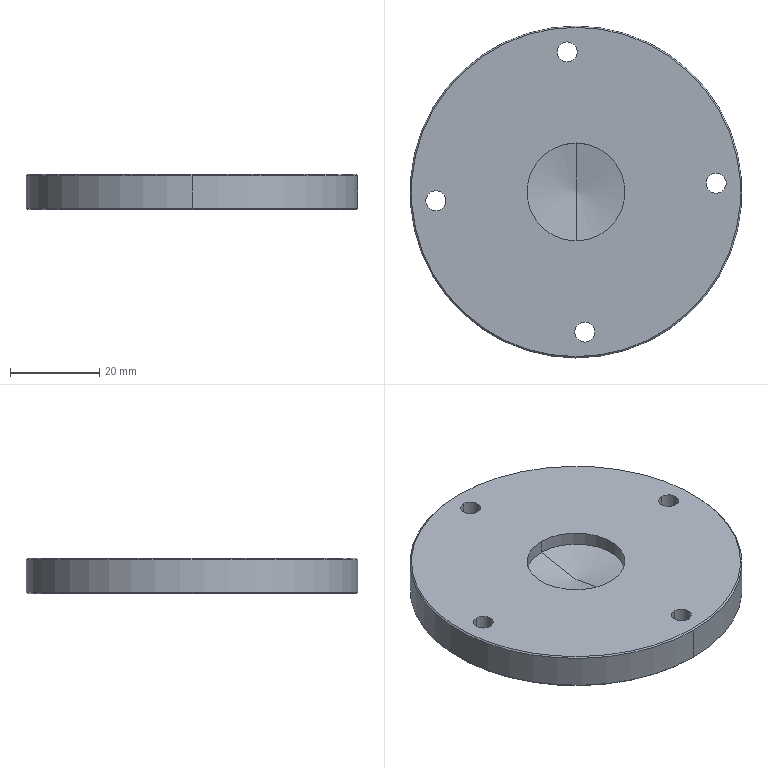Part | SolidWorks | features BaseBody 1 | 1 solid | 32 faces | box 74.5 x 74.5 x 8 mm | volume 32380 mm3 | cylinder 20 | cone 6 | plane 6 | commonest cylinder face diameters 4.5 x8 8 x8 22 x2 74.5 x2
STEP:
#1=CARTESIAN_POINT('',(560.081,-185.625,38.889));
#2=VERTEX_POINT('',#1);
#3=CARTESIAN_POINT('',(560.081,-193.625,38.889));
#4=VERTEX_POINT('',#3);
#5=CARTESIAN_POINT('',(560.081,-189.625,38.889));
#6=DIRECTION('',(0.,-0.000000003,1.));
#7=DIRECTION('',(0.,-1.,-0.000000003));
#8=AXIS2_PLACEMENT_3D('',#5,#6,#7);
#9=CIRCLE('',#8,4.);
#10=EDGE_CURVE('',#2,#4,#9,.T.);
#11=ORIENTED_EDGE('',*,*,#10,.F.);
#12=CARTESIAN_POINT('',(560.081,-185.625,43.089));
#13=VERTEX_POINT('',#12);
#14=CARTESIAN_POINT('',(560.081,-185.625,38.889));
#15=DIRECTION('',(0.,-0.000000003,1.));
#16=VECTOR('',#15,1000.);
#17=LINE('',#14,#16);
#18=EDGE_CURVE('',#2,#13,#17,.T.);
#19=ORIENTED_EDGE('',*,*,#18,.T.);
#20=CARTESIAN_POINT('',(560.081,-193.625,43.089));
#21=VERTEX_POINT('',#20);
#22=CARTESIAN_POINT('',(560.081,-189.625,43.089));
#23=DIRECTION('',(0.,0.000000003,-1.));
#24=DIRECTION('',(0.,-1.,-0.000000003));
#25=AXIS2_PLACEMENT_3D('',#22,#23,#24);
#26=CIRCLE('',#25,4.);
#27=EDGE_CURVE('',#21,#13,#26,.T.);
#28=ORIENTED_EDGE('',*,*,#27,.F.);
#29=CARTESIAN_POINT('',(560.081,-193.625,38.889));
#30=DIRECTION('',(0.,-0.000000003,1.));
#31=VECTOR('',#30,1000.);
#32=LINE('',#29,#31);
#33=EDGE_CURVE('',#4,#21,#32,.T.);
#34=ORIENTED_EDGE('',*,*,#33,.F.);
#35=EDGE_LOOP('',(#11,#19,#28,#34));
#36=FACE_OUTER_BOUND('',#35,.T.);
#37=CARTESIAN_POINT('',(560.081,-189.625,38.889));
#38=DIRECTION('',(0.,-0.000000003,1.));
#39=DIRECTION('',(0.,-1.,-0.000000003));
#40=AXIS2_PLACEMENT_3D('',#37,#38,#39);
#41=CYLINDRICAL_SURFACE('',#40,4.);
#42=ADVANCED_FACE('',(#36),#41,.F.);
#43=CARTESIAN_POINT('',(593.495,-215.086,38.889));
#44=VERTEX_POINT('',#43);
#45=CARTESIAN_POINT('',(593.495,-223.086,38.889));
#46=VERTEX_POINT('',#45);
#47=CARTESIAN_POINT('',(593.495,-219.086,38.889));
#48=DIRECTION('',(0.,-0.000000003,1.));
#49=DIRECTION('',(0.,-1.,-0.000000003));
#50=AXIS2_PLACEMENT_3D('',#47,#48,#49);
#51=CIRCLE('',#50,4.);
#52=EDGE_CURVE('',#44,#46,#51,.T.);
#53=ORIENTED_EDGE('',*,*,#52,.F.);
#54=CARTESIAN_POINT('',(593.495,-215.086,43.089));
#55=VERTEX_POINT('',#54);
#56=CARTESIAN_POINT('',(593.495,-215.086,38.889));
#57=DIRECTION('',(0.,-0.000000003,1.));
#58=VECTOR('',#57,1000.);
#59=LINE('',#56,#58);
#60=EDGE_CURVE('',#44,#55,#59,.T.);
#61=ORIENTED_EDGE('',*,*,#60,.T.);
#62=CARTESIAN_POINT('',(593.495,-223.086,43.089));
#63=VERTEX_POINT('',#62);
#64=CARTESIAN_POINT('',(593.495,-219.086,43.089));
#65=DIRECTION('',(0.,0.000000003,-1.));
#66=DIRECTION('',(0.,-1.,-0.000000003));
#67=AXIS2_PLACEMENT_3D('',#64,#65,#66);
#68=CIRCLE('',#67,4.);
#69=EDGE_CURVE('',#63,#55,#68,.T.);
#70=ORIENTED_EDGE('',*,*,#69,.F.);
#71=CARTESIAN_POINT('',(593.495,-223.086,38.889));
#72=DIRECTION('',(0.,-0.000000003,1.));
#73=VECTOR('',#72,1000.);
#74=LINE('',#71,#73);
#75=EDGE_CURVE('',#46,#63,#74,.T.);
#76=ORIENTED_EDGE('',*,*,#75,.F.);
#77=EDGE_LOOP('',(#53,#61,#70,#76));
#78=FACE_OUTER_BOUND('',#77,.T.);
#79=CARTESIAN_POINT('',(593.495,-219.086,38.889));
#80=DIRECTION('',(0.,-0.000000003,1.));
#81=DIRECTION('',(0.,-1.,-0.000000003));
#82=AXIS2_PLACEMENT_3D('',#79,#80,#81);
#83=CYLINDRICAL_SURFACE('',#82,4.);
#84=ADVANCED_FACE('',(#78),#83,.F.);
#85=CARTESIAN_POINT('',(622.957,-181.672,38.889));
#86=VERTEX_POINT('',#85);
#87=CARTESIAN_POINT('',(622.957,-189.672,38.889));
#88=VERTEX_POINT('',#87);
#89=CARTESIAN_POINT('',(622.957,-185.672,38.889));
#90=DIRECTION('',(0.,-0.000000003,1.));
#91=DIRECTION('',(0.,-1.,-0.000000003));
#92=AXIS2_PLACEMENT_3D('',#89,#90,#91);
#93=CIRCLE('',#92,4.);
#94=EDGE_CURVE('',#86,#88,#93,.T.);
#95=ORIENTED_EDGE('',*,*,#94,.F.);
#96=CARTESIAN_POINT('',(622.957,-181.672,43.089));
#97=VERTEX_POINT('',#96);
#98=CARTESIAN_POINT('',(622.957,-181.672,38.889));
#99=DIRECTION('',(0.,-0.000000003,1.));
#100=VECTOR('',#99,1000.);
#101=LINE('',#98,#100);
#102=EDGE_CURVE('',#86,#97,#101,.T.);
#103=ORIENTED_EDGE('',*,*,#102,.T.);
#104=CARTESIAN_POINT('',(622.957,-189.672,43.089));
#105=VERTEX_POINT('',#104);
#106=CARTESIAN_POINT('',(622.957,-185.672,43.089));
#107=DIRECTION('',(0.,0.000000003,-1.));
#108=DIRECTION('',(0.,-1.,-0.000000003));
#109=AXIS2_PLACEMENT_3D('',#106,#107,#108);
#110=CIRCLE('',#109,4.);
#111=EDGE_CURVE('',#105,#97,#110,.T.);
#112=ORIENTED_EDGE('',*,*,#111,.F.);
#113=CARTESIAN_POINT('',(622.957,-189.672,38.889));
#114=DIRECTION('',(0.,-0.000000003,1.));
#115=VECTOR('',#114,1000.);
#116=LINE('',#113,#115);
#117=EDGE_CURVE('',#88,#105,#116,.T.);
#118=ORIENTED_EDGE('',*,*,#117,.F.);
#119=EDGE_LOOP('',(#95,#103,#112,#118));
#120=FACE_OUTER_BOUND('',#119,.T.);
#121=CARTESIAN_POINT('',(622.957,-185.672,38.889));
#122=DIRECTION('',(0.,-0.000000003,1.));
#123=DIRECTION('',(0.,-1.,-0.000000003));
#124=AXIS2_PLACEMENT_3D('',#121,#122,#123);
#125=CYLINDRICAL_SURFACE('',#124,4.);
#126=ADVANCED_FACE('',(#120),#125,.F.);
#127=CARTESIAN_POINT('',(589.542,-152.21,38.889));
#128=VERTEX_POINT('',#127);
#129=CARTESIAN_POINT('',(589.542,-160.21,38.889));
#130=VERTEX_POINT('',#129);
#131=CARTESIAN_POINT('',(589.542,-156.21,38.889));
#132=DIRECTION('',(0.,-0.000000003,1.));
#133=DIRECTION('',(0.,-1.,-0.000000003));
#134=AXIS2_PLACEMENT_3D('',#131,#132,#133);
#135=CIRCLE('',#134,4.);
#136=EDGE_CURVE('',#128,#130,#135,.T.);
#137=ORIENTED_EDGE('',*,*,#136,.F.);
#138=CARTESIAN_POINT('',(589.542,-152.21,43.089));
#139=VERTEX_POINT('',#138);
#140=CARTESIAN_POINT('',(589.542,-152.21,38.889));
#141=DIRECTION('',(0.,-0.000000003,1.));
#142=VECTOR('',#141,1000.);
#143=LINE('',#140,#142);
#144=EDGE_CURVE('',#128,#139,#143,.T.);
#145=ORIENTED_EDGE('',*,*,#144,.T.);
#146=CARTESIAN_POINT('',(589.542,-160.21,43.089));
#147=VERTEX_POINT('',#146);
#148=CARTESIAN_POINT('',(589.542,-156.21,43.089));
#149=DIRECTION('',(0.,0.000000003,-1.));
#150=DIRECTION('',(0.,-1.,-0.000000003));
#151=AXIS2_PLACEMENT_3D('',#148,#149,#150);
#152=CIRCLE('',#151,4.);
#153=EDGE_CURVE('',#147,#139,#152,.T.);
#154=ORIENTED_EDGE('',*,*,#153,.F.);
#155=CARTESIAN_POINT('',(589.542,-160.21,38.889));
#156=DIRECTION('',(0.,-0.000000003,1.));
#157=VECTOR('',#156,1000.);
#158=LINE('',#155,#157);
#159=EDGE_CURVE('',#130,#147,#158,.T.);
#160=ORIENTED_EDGE('',*,*,#159,.F.);
#161=EDGE_LOOP('',(#137,#145,#154,#160));
#162=FACE_OUTER_BOUND('',#161,.T.);
#163=CARTESIAN_POINT('',(589.542,-156.21,38.889));
#164=DIRECTION('',(0.,-0.000000003,1.));
#165=DIRECTION('',(0.,-1.,-0.000000003));
#166=AXIS2_PLACEMENT_3D('',#163,#164,#165);
#167=CYLINDRICAL_SURFACE('',#166,4.);
#168=ADVANCED_FACE('',(#162),#167,.F.);
#169=CARTESIAN_POINT('',(591.519,-150.698,38.889));
#170=VERTEX_POINT('',#169);
#171=CARTESIAN_POINT('',(591.519,-224.598,38.889));
#172=VERTEX_POINT('',#171);
#173=CARTESIAN_POINT('',(591.519,-187.648,38.889));
#174=DIRECTION('',(0.,0.000000003,-1.));
#175=DIRECTION('',(0.,-1.,-0.000000003));
#176=AXIS2_PLACEMENT_3D('',#173,#174,#175);
#177=CIRCLE('',#176,36.95);
#178=EDGE_CURVE('',#170,#172,#177,.T.);
#179=ORIENTED_EDGE('',*,*,#178,.F.);
#180=CARTESIAN_POINT('',(591.519,-150.398,39.189));
#181=VERTEX_POINT('',#180);
#182=CARTESIAN_POINT('',(591.519,-150.398,39.189));
#183=DIRECTION('',(0.,0.7071,0.7071));
#184=VECTOR('',#183,1000.);
#185=LINE('',#182,#184);
#186=EDGE_CURVE('',#170,#181,#185,.T.);
#187=ORIENTED_EDGE('',*,*,#186,.T.);
#188=CARTESIAN_POINT('',(591.519,-224.898,39.189));
#189=VERTEX_POINT('',#188);
#190=CARTESIAN_POINT('',(591.519,-187.648,39.189));
#191=DIRECTION('',(0.,0.000000003,-1.));
#192=DIRECTION('',(-0.998,-0.06274,0.));
#193=AXIS2_PLACEMENT_3D('',#190,#191,#192);
#194=CIRCLE('',#193,37.25);
#195=EDGE_CURVE('',#181,#189,#194,.T.);
#196=ORIENTED_EDGE('',*,*,#195,.T.);
#197=CARTESIAN_POINT('',(591.519,-224.898,39.189));
#198=DIRECTION('',(0.,-0.7071,0.7071));
#199=VECTOR('',#198,1000.);
#200=LINE('',#197,#199);
#201=EDGE_CURVE('',#172,#189,#200,.T.);
#202=ORIENTED_EDGE('',*,*,#201,.F.);
#203=EDGE_LOOP('',(#179,#187,#196,#202));
#204=FACE_OUTER_BOUND('',#203,.T.);
#205=CARTESIAN_POINT('',(591.519,-187.648,39.189));
#206=DIRECTION('',(0.,-0.000000003,1.));
#207=DIRECTION('',(0.,-1.,-0.000000003));
#208=AXIS2_PLACEMENT_3D('',#205,#206,#207);
#209=CONICAL_SURFACE('',#208,37.25,0.7854);
#210=ADVANCED_FACE('',(#204),#209,.T.);
#211=ORIENTED_EDGE('',*,*,#195,.F.);
#212=CARTESIAN_POINT('',(591.519,-150.398,46.589));
#213=VERTEX_POINT('',#212);
#214=CARTESIAN_POINT('',(591.519,-150.398,38.489));
#215=DIRECTION('',(0.,-0.000000003,1.));
#216=VECTOR('',#215,1000.);
#217=LINE('',#214,#216);
#218=EDGE_CURVE('',#181,#213,#217,.T.);
#219=ORIENTED_EDGE('',*,*,#218,.T.);
#220=CARTESIAN_POINT('',(591.519,-224.898,46.589));
#221=VERTEX_POINT('',#220);
#222=CARTESIAN_POINT('',(591.519,-187.648,46.589));
#223=DIRECTION('',(0.,0.000000003,-1.));
#224=DIRECTION('',(0.,-1.,-0.000000003));
#225=AXIS2_PLACEMENT_3D('',#222,#223,#224);
#226=CIRCLE('',#225,37.25);
#227=EDGE_CURVE('',#213,#221,#226,.T.);
#228=ORIENTED_EDGE('',*,*,#227,.T.);
#229=CARTESIAN_POINT('',(591.519,-224.898,38.489));
#230=DIRECTION('',(0.,-0.000000003,1.));
#231=VECTOR('',#230,1000.);
#232=LINE('',#229,#231);
#233=EDGE_CURVE('',#189,#221,#232,.T.);
#234=ORIENTED_EDGE('',*,*,#233,.F.);
#235=EDGE_LOOP('',(#211,#219,#228,#234));
#236=FACE_OUTER_BOUND('',#235,.T.);
#237=CARTESIAN_POINT('',(591.519,-187.648,38.489));
#238=DIRECTION('',(0.,-0.000000003,1.));
#239=DIRECTION('',(0.,-1.,-0.000000003));
#240=AXIS2_PLACEMENT_3D('',#237,#238,#239);
#241=CYLINDRICAL_SURFACE('',#240,37.25);
#242=ADVANCED_FACE('',(#236),#241,.T.);
#243=CARTESIAN_POINT('',(560.081,-187.375,43.089));
#244=VERTEX_POINT('',#243);
#245=CARTESIAN_POINT('',(560.081,-191.875,43.089));
#246=VERTEX_POINT('',#245);
#247=CARTESIAN_POINT('',(560.081,-189.625,43.089));
#248=DIRECTION('',(0.,-0.000000003,1.));
#249=DIRECTION('',(0.,-1.,-0.000000003));
#250=AXIS2_PLACEMENT_3D('',#247,#248,#249);
#251=CIRCLE('',#250,2.25);
#252=EDGE_CURVE('',#244,#246,#251,.T.);
#253=ORIENTED_EDGE('',*,*,#252,.F.);
#254=CARTESIAN_POINT('',(560.081,-187.375,46.889));
#255=VERTEX_POINT('',#254);
#256=CARTESIAN_POINT('',(560.081,-187.375,38.889));
#257=DIRECTION('',(0.,-0.000000003,1.));
#258=VECTOR('',#257,1000.);
#259=LINE('',#256,#258);
#260=EDGE_CURVE('',#244,#255,#259,.T.);
#261=ORIENTED_EDGE('',*,*,#260,.T.);
#262=CARTESIAN_POINT('',(560.081,-191.875,46.889));
#263=VERTEX_POINT('',#262);
#264=CARTESIAN_POINT('',(560.081,-189.625,46.889));
#265=DIRECTION('',(0.,0.000000003,-1.));
#266=DIRECTION('',(0.,-1.,-0.000000003));
#267=AXIS2_PLACEMENT_3D('',#264,#265,#266);
#268=CIRCLE('',#267,2.25);
#269=EDGE_CURVE('',#263,#255,#268,.T.);
#270=ORIENTED_EDGE('',*,*,#269,.F.);
#271=CARTESIAN_POINT('',(560.081,-191.875,38.889));
#272=DIRECTION('',(0.,-0.000000003,1.));
#273=VECTOR('',#272,1000.);
#274=LINE('',#271,#273);
#275=EDGE_CURVE('',#246,#263,#274,.T.);
#276=ORIENTED_EDGE('',*,*,#275,.F.);
#277=EDGE_LOOP('',(#253,#261,#270,#276));
#278=FACE_OUTER_BOUND('',#277,.T.);
#279=CARTESIAN_POINT('',(560.081,-189.625,38.889));
#280=DIRECTION('',(0.,-0.000000003,1.));
#281=DIRECTION('',(0.,-1.,-0.000000003));
#282=AXIS2_PLACEMENT_3D('',#279,#280,#281);
#283=CYLINDRICAL_SURFACE('',#282,2.25);
#284=ADVANCED_FACE('',(#278),#283,.F.);
#285=CARTESIAN_POINT('',(593.495,-216.836,43.089));
#286=VERTEX_POINT('',#285);
#287=CARTESIAN_POINT('',(593.495,-221.336,43.089));
#288=VERTEX_POINT('',#287);
#289=CARTESIAN_POINT('',(593.495,-219.086,43.089));
#290=DIRECTION('',(0.,-0.000000003,1.));
#291=DIRECTION('',(0.,-1.,-0.000000003));
#292=AXIS2_PLACEMENT_3D('',#289,#290,#291);
#293=CIRCLE('',#292,2.25);
#294=EDGE_CURVE('',#286,#288,#293,.T.);
#295=ORIENTED_EDGE('',*,*,#294,.F.);
#296=CARTESIAN_POINT('',(593.495,-216.836,46.889));
#297=VERTEX_POINT('',#296);
#298=CARTESIAN_POINT('',(593.495,-216.836,38.889));
#299=DIRECTION('',(0.,-0.000000003,1.));
#300=VECTOR('',#299,1000.);
#301=LINE('',#298,#300);
#302=EDGE_CURVE('',#286,#297,#301,.T.);
#303=ORIENTED_EDGE('',*,*,#302,.T.);
#304=CARTESIAN_POINT('',(593.495,-221.336,46.889));
#305=VERTEX_POINT('',#304);
#306=CARTESIAN_POINT('',(593.495,-219.086,46.889));
#307=DIRECTION('',(0.,0.000000003,-1.));
#308=DIRECTION('',(0.,-1.,-0.000000003));
#309=AXIS2_PLACEMENT_3D('',#306,#307,#308);
#310=CIRCLE('',#309,2.25);
#311=EDGE_CURVE('',#305,#297,#310,.T.);
#312=ORIENTED_EDGE('',*,*,#311,.F.);
#313=CARTESIAN_POINT('',(593.495,-221.336,38.889));
#314=DIRECTION('',(0.,-0.000000003,1.));
#315=VECTOR('',#314,1000.);
#316=LINE('',#313,#315);
#317=EDGE_CURVE('',#288,#305,#316,.T.);
#318=ORIENTED_EDGE('',*,*,#317,.F.);
#319=EDGE_LOOP('',(#295,#303,#312,#318));
#320=FACE_OUTER_BOUND('',#319,.T.);
#321=CARTESIAN_POINT('',(593.495,-219.086,38.889));
#322=DIRECTION('',(0.,-0.000000003,1.));
#323=DIRECTION('',(0.,-1.,-0.000000003));
#324=AXIS2_PLACEMENT_3D('',#321,#322,#323);
#325=CYLINDRICAL_SURFACE('',#324,2.25);
#326=ADVANCED_FACE('',(#320),#325,.F.);
#327=CARTESIAN_POINT('',(622.957,-183.422,43.089));
#328=VERTEX_POINT('',#327);
#329=CARTESIAN_POINT('',(622.957,-187.922,43.089));
#330=VERTEX_POINT('',#329);
#331=CARTESIAN_POINT('',(622.957,-185.672,43.089));
#332=DIRECTION('',(0.,-0.000000003,1.));
#333=DIRECTION('',(0.,-1.,-0.000000003));
#334=AXIS2_PLACEMENT_3D('',#331,#332,#333);
#335=CIRCLE('',#334,2.25);
#336=EDGE_CURVE('',#328,#330,#335,.T.);
#337=ORIENTED_EDGE('',*,*,#336,.F.);
#338=CARTESIAN_POINT('',(622.957,-183.422,46.889));
#339=VERTEX_POINT('',#338);
#340=CARTESIAN_POINT('',(622.957,-183.422,38.889));
#341=DIRECTION('',(0.,-0.000000003,1.));
#342=VECTOR('',#341,1000.);
#343=LINE('',#340,#342);
#344=EDGE_CURVE('',#328,#339,#343,.T.);
#345=ORIENTED_EDGE('',*,*,#344,.T.);
#346=CARTESIAN_POINT('',(622.957,-187.922,46.889));
#347=VERTEX_POINT('',#346);
#348=CARTESIAN_POINT('',(622.957,-185.672,46.889));
#349=DIRECTION('',(0.,0.000000003,-1.));
#350=DIRECTION('',(0.,-1.,-0.000000003));
#351=AXIS2_PLACEMENT_3D('',#348,#349,#350);
#352=CIRCLE('',#351,2.25);
#353=EDGE_CURVE('',#347,#339,#352,.T.);
#354=ORIENTED_EDGE('',*,*,#353,.F.);
#355=CARTESIAN_POINT('',(622.957,-187.922,38.889));
#356=DIRECTION('',(0.,-0.000000003,1.));
#357=VECTOR('',#356,1000.);
#358=LINE('',#355,#357);
#359=EDGE_CURVE('',#330,#347,#358,.T.);
#360=ORIENTED_EDGE('',*,*,#359,.F.);
#361=EDGE_LOOP('',(#337,#345,#354,#360));
#362=FACE_OUTER_BOUND('',#361,.T.);
#363=CARTESIAN_POINT('',(622.957,-185.672,38.889));
#364=DIRECTION('',(0.,-0.000000003,1.));
#365=DIRECTION('',(0.,-1.,-0.000000003));
#366=AXIS2_PLACEMENT_3D('',#363,#364,#365);
#367=CYLINDRICAL_SURFACE('',#366,2.25);
#368=ADVANCED_FACE('',(#362),#367,.F.);
#369=CARTESIAN_POINT('',(589.542,-153.96,43.089));
#370=VERTEX_POINT('',#369);
#371=CARTESIAN_POINT('',(589.542,-158.46,43.089));
#372=VERTEX_POINT('',#371);
#373=CARTESIAN_POINT('',(589.542,-156.21,43.089));
#374=DIRECTION('',(0.,-0.000000003,1.));
#375=DIRECTION('',(0.,-1.,-0.000000003));
#376=AXIS2_PLACEMENT_3D('',#373,#374,#375);
#377=CIRCLE('',#376,2.25);
#378=EDGE_CURVE('',#370,#372,#377,.T.);
#379=ORIENTED_EDGE('',*,*,#378,.F.);
#380=CARTESIAN_POINT('',(589.542,-153.96,46.889));
#381=VERTEX_POINT('',#380);
#382=CARTESIAN_POINT('',(589.542,-153.96,38.889));
#383=DIRECTION('',(0.,-0.000000003,1.));
#384=VECTOR('',#383,1000.);
#385=LINE('',#382,#384);
#386=EDGE_CURVE('',#370,#381,#385,.T.);
#387=ORIENTED_EDGE('',*,*,#386,.T.);
#388=CARTESIAN_POINT('',(589.542,-158.46,46.889));
#389=VERTEX_POINT('',#388);
#390=CARTESIAN_POINT('',(589.542,-156.21,46.889));
#391=DIRECTION('',(0.,0.000000003,-1.));
#392=DIRECTION('',(0.,-1.,-0.000000003));
#393=AXIS2_PLACEMENT_3D('',#390,#391,#392);
#394=CIRCLE('',#393,2.25);
#395=EDGE_CURVE('',#389,#381,#394,.T.);
#396=ORIENTED_EDGE('',*,*,#395,.F.);
#397=CARTESIAN_POINT('',(589.542,-158.46,38.889));
#398=DIRECTION('',(0.,-0.000000003,1.));
#399=VECTOR('',#398,1000.);
#400=LINE('',#397,#399);
#401=EDGE_CURVE('',#372,#389,#400,.T.);
#402=ORIENTED_EDGE('',*,*,#401,.F.);
#403=EDGE_LOOP('',(#379,#387,#396,#402));
#404=FACE_OUTER_BOUND('',#403,.T.);
#405=CARTESIAN_POINT('',(589.542,-156.21,38.889));
#406=DIRECTION('',(0.,-0.000000003,1.));
#407=DIRECTION('',(0.,-1.,-0.000000003));
#408=AXIS2_PLACEMENT_3D('',#405,#406,#407);
#409=CYLINDRICAL_SURFACE('',#408,2.25);
#410=ADVANCED_FACE('',(#404),#409,.F.);
#411=CARTESIAN_POINT('',(591.519,-150.698,46.889));
#412=VERTEX_POINT('',#411);
#413=CARTESIAN_POINT('',(591.519,-224.598,46.889));
#414=VERTEX_POINT('',#413);
#415=CARTESIAN_POINT('',(591.519,-187.648,46.889));
#416=DIRECTION('',(0.,0.000000003,-1.));
#417=DIRECTION('',(0.,1.,0.000000003));
#418=AXIS2_PLACEMENT_3D('',#415,#416,#417);
#419=CIRCLE('',#418,36.95);
#420=EDGE_CURVE('',#412,#414,#419,.T.);
#421=ORIENTED_EDGE('',*,*,#420,.T.);
#422=CARTESIAN_POINT('',(591.519,-224.898,46.589));
#423=DIRECTION('',(0.,-0.7071,-0.7071));
#424=VECTOR('',#423,1000.);
#425=LINE('',#422,#424);
#426=EDGE_CURVE('',#414,#221,#425,.T.);
#427=ORIENTED_EDGE('',*,*,#426,.T.);
#428=ORIENTED_EDGE('',*,*,#227,.F.);
#429=CARTESIAN_POINT('',(591.519,-150.398,46.589));
#430=DIRECTION('',(0.,0.7071,-0.7071));
#431=VECTOR('',#430,1000.);
#432=LINE('',#429,#431);
#433=EDGE_CURVE('',#412,#213,#432,.T.);
#434=ORIENTED_EDGE('',*,*,#433,.F.);
#435=EDGE_LOOP('',(#421,#427,#428,#434));
#436=FACE_OUTER_BOUND('',#435,.T.);
#437=CARTESIAN_POINT('',(591.519,-187.648,46.589));
#438=DIRECTION('',(0.,0.000000003,-1.));
#439=DIRECTION('',(0.,1.,0.000000003));
#440=AXIS2_PLACEMENT_3D('',#437,#438,#439);
#441=CONICAL_SURFACE('',#440,37.25,0.7854);
#442=ADVANCED_FACE('',(#436),#441,.T.);
#443=CARTESIAN_POINT('',(591.519,-176.648,43.889));
#444=VERTEX_POINT('',#443);
#445=CARTESIAN_POINT('',(591.519,-198.648,43.889));
#446=VERTEX_POINT('',#445);
#447=CARTESIAN_POINT('',(591.519,-187.648,43.889));
#448=DIRECTION('',(0.,-0.000000003,1.));
#449=DIRECTION('',(0.,-1.,-0.000000003));
#450=AXIS2_PLACEMENT_3D('',#447,#448,#449);
#451=CIRCLE('',#450,11.);
#452=EDGE_CURVE('',#444,#446,#451,.T.);
#453=ORIENTED_EDGE('',*,*,#452,.F.);
#454=CARTESIAN_POINT('',(591.519,-176.648,46.889));
#455=VERTEX_POINT('',#454);
#456=CARTESIAN_POINT('',(591.519,-176.648,38.489));
#457=DIRECTION('',(0.,-0.000000003,1.));
#458=VECTOR('',#457,1000.);
#459=LINE('',#456,#458);
#460=EDGE_CURVE('',#444,#455,#459,.T.);
#461=ORIENTED_EDGE('',*,*,#460,.T.);
#462=CARTESIAN_POINT('',(591.519,-198.648,46.889));
#463=VERTEX_POINT('',#462);
#464=CARTESIAN_POINT('',(591.519,-187.648,46.889));
#465=DIRECTION('',(0.,-0.000000003,1.));
#466=DIRECTION('',(0.,-1.,-0.000000003));
#467=AXIS2_PLACEMENT_3D('',#464,#465,#466);
#468=CIRCLE('',#467,11.);
#469=EDGE_CURVE('',#455,#463,#468,.T.);
#470=ORIENTED_EDGE('',*,*,#469,.T.);
#471=CARTESIAN_POINT('',(591.519,-198.648,38.489));
#472=DIRECTION('',(0.,-0.000000003,1.));
#473=VECTOR('',#472,1000.);
#474=LINE('',#471,#473);
#475=EDGE_CURVE('',#446,#463,#474,.T.);
#476=ORIENTED_EDGE('',*,*,#475,.F.);
#477=EDGE_LOOP('',(#453,#461,#470,#476));
#478=FACE_OUTER_BOUND('',#477,.T.);
#479=CARTESIAN_POINT('',(591.519,-187.648,38.489));
#480=DIRECTION('',(0.,-0.000000003,1.));
#481=DIRECTION('',(0.,-1.,-0.000000003));
#482=AXIS2_PLACEMENT_3D('',#479,#480,#481);
#483=CYLINDRICAL_SURFACE('',#482,11.);
#484=ADVANCED_FACE('',(#478),#483,.F.);
#485=CARTESIAN_POINT('',(591.519,-187.648,41.949));
#486=VERTEX_POINT('',#485);
#487=CARTESIAN_POINT('',(591.519,-198.648,43.889));
#488=DIRECTION('',(0.,-0.9848,0.1736));
#489=VECTOR('',#488,1000.);
#490=LINE('',#487,#489);
#491=EDGE_CURVE('',#486,#446,#490,.T.);
#492=ORIENTED_EDGE('',*,*,#491,.F.);
#493=CARTESIAN_POINT('',(591.519,-176.648,43.889));
#494=DIRECTION('',(0.,0.9848,0.1736));
#495=VECTOR('',#494,1000.);
#496=LINE('',#493,#495);
#497=EDGE_CURVE('',#486,#444,#496,.T.);
#498=ORIENTED_EDGE('',*,*,#497,.T.);
#499=ORIENTED_EDGE('',*,*,#452,.T.);
#500=EDGE_LOOP('',(#492,#498,#499));
#501=FACE_OUTER_BOUND('',#500,.T.);
#502=CARTESIAN_POINT('',(591.519,-187.648,43.889));
#503=DIRECTION('',(0.,-0.000000003,1.));
#504=DIRECTION('',(0.,-1.,-0.000000003));
#505=AXIS2_PLACEMENT_3D('',#502,#503,#504);
#506=CONICAL_SURFACE('',#505,11.,1.396);
#507=ADVANCED_FACE('',(#501),#506,.F.);
#508=CARTESIAN_POINT('',(560.081,-189.625,38.889));
#509=DIRECTION('',(0.,-0.000000003,1.));
#510=DIRECTION('',(0.,-1.,-0.000000003));
#511=AXIS2_PLACEMENT_3D('',#508,#509,#510);
#512=CIRCLE('',#511,4.);
#513=EDGE_CURVE('',#4,#2,#512,.T.);
#514=ORIENTED_EDGE('',*,*,#513,.T.);
#515=ORIENTED_EDGE('',*,*,#10,.T.);
#516=EDGE_LOOP('',(#514,#515));
#517=FACE_BOUND('',#516,.T.);
#518=CARTESIAN_POINT('',(593.495,-219.086,38.889));
#519=DIRECTION('',(0.,-0.000000003,1.));
#520=DIRECTION('',(0.,-1.,-0.000000003));
#521=AXIS2_PLACEMENT_3D('',#518,#519,#520);
#522=CIRCLE('',#521,4.);
#523=EDGE_CURVE('',#46,#44,#522,.T.);
#524=ORIENTED_EDGE('',*,*,#523,.T.);
#525=ORIENTED_EDGE('',*,*,#52,.T.);
#526=EDGE_LOOP('',(#524,#525));
#527=FACE_BOUND('',#526,.T.);
#528=CARTESIAN_POINT('',(622.957,-185.672,38.889));
#529=DIRECTION('',(0.,-0.000000003,1.));
#530=DIRECTION('',(0.,-1.,-0.000000003));
#531=AXIS2_PLACEMENT_3D('',#528,#529,#530);
#532=CIRCLE('',#531,4.);
#533=EDGE_CURVE('',#88,#86,#532,.T.);
#534=ORIENTED_EDGE('',*,*,#533,.T.);
#535=ORIENTED_EDGE('',*,*,#94,.T.);
#536=EDGE_LOOP('',(#534,#535));
#537=FACE_BOUND('',#536,.T.);
#538=CARTESIAN_POINT('',(589.542,-156.21,38.889));
#539=DIRECTION('',(0.,-0.000000003,1.));
#540=DIRECTION('',(0.,-1.,-0.000000003));
#541=AXIS2_PLACEMENT_3D('',#538,#539,#540);
#542=CIRCLE('',#541,4.);
#543=EDGE_CURVE('',#130,#128,#542,.T.);
#544=ORIENTED_EDGE('',*,*,#543,.T.);
#545=ORIENTED_EDGE('',*,*,#136,.T.);
#546=EDGE_LOOP('',(#544,#545));
#547=FACE_BOUND('',#546,.T.);
#548=CARTESIAN_POINT('',(591.519,-187.648,38.889));
#549=DIRECTION('',(0.,0.000000003,-1.));
#550=DIRECTION('',(0.,-1.,-0.000000003));
#551=AXIS2_PLACEMENT_3D('',#548,#549,#550);
#552=CIRCLE('',#551,36.95);
#553=EDGE_CURVE('',#172,#170,#552,.T.);
#554=ORIENTED_EDGE('',*,*,#553,.T.);
#555=ORIENTED_EDGE('',*,*,#178,.T.);
#556=EDGE_LOOP('',(#554,#555));
#557=FACE_OUTER_BOUND('',#556,.T.);
#558=CARTESIAN_POINT('',(591.519,-187.648,38.889));
#559=DIRECTION('',(0.,0.000000003,-1.));
#560=DIRECTION('',(0.,1.,0.000000003));
#561=AXIS2_PLACEMENT_3D('',#558,#559,#560);
#562=PLANE('',#561);
#563=ADVANCED_FACE('',(#517,#527,#537,#547,#557),#562,.T.);
#564=ORIENTED_EDGE('',*,*,#18,.F.);
#565=ORIENTED_EDGE('',*,*,#513,.F.);
#566=ORIENTED_EDGE('',*,*,#33,.T.);
#567=CARTESIAN_POINT('',(560.081,-189.625,43.089));
#568=DIRECTION('',(0.,0.000000003,-1.));
#569=DIRECTION('',(0.,-1.,-0.000000003));
#570=AXIS2_PLACEMENT_3D('',#567,#568,#569);
#571=CIRCLE('',#570,4.);
#572=EDGE_CURVE('',#13,#21,#571,.T.);
#573=ORIENTED_EDGE('',*,*,#572,.F.);
#574=EDGE_LOOP('',(#564,#565,#566,#573));
#575=FACE_OUTER_BOUND('',#574,.T.);
#576=CARTESIAN_POINT('',(560.081,-189.625,38.889));
#577=DIRECTION('',(0.,-0.000000003,1.));
#578=DIRECTION('',(0.,-1.,-0.000000003));
#579=AXIS2_PLACEMENT_3D('',#576,#577,#578);
#580=CYLINDRICAL_SURFACE('',#579,4.);
#581=ADVANCED_FACE('',(#575),#580,.F.);
#582=ORIENTED_EDGE('',*,*,#60,.F.);
#583=ORIENTED_EDGE('',*,*,#523,.F.);
#584=ORIENTED_EDGE('',*,*,#75,.T.);
#585=CARTESIAN_POINT('',(593.495,-219.086,43.089));
#586=DIRECTION('',(0.,0.000000003,-1.));
#587=DIRECTION('',(0.,-1.,-0.000000003));
#588=AXIS2_PLACEMENT_3D('',#585,#586,#587);
#589=CIRCLE('',#588,4.);
#590=EDGE_CURVE('',#55,#63,#589,.T.);
#591=ORIENTED_EDGE('',*,*,#590,.F.);
#592=EDGE_LOOP('',(#582,#583,#584,#591));
#593=FACE_OUTER_BOUND('',#592,.T.);
#594=CARTESIAN_POINT('',(593.495,-219.086,38.889));
#595=DIRECTION('',(0.,-0.000000003,1.));
#596=DIRECTION('',(0.,-1.,-0.000000003));
#597=AXIS2_PLACEMENT_3D('',#594,#595,#596);
#598=CYLINDRICAL_SURFACE('',#597,4.);
#599=ADVANCED_FACE('',(#593),#598,.F.);
#600=ORIENTED_EDGE('',*,*,#102,.F.);
#601=ORIENTED_EDGE('',*,*,#533,.F.);
#602=ORIENTED_EDGE('',*,*,#117,.T.);
#603=CARTESIAN_POINT('',(622.957,-185.672,43.089));
#604=DIRECTION('',(0.,0.000000003,-1.));
#605=DIRECTION('',(0.,-1.,-0.000000003));
#606=AXIS2_PLACEMENT_3D('',#603,#604,#605);
#607=CIRCLE('',#606,4.);
#608=EDGE_CURVE('',#97,#105,#607,.T.);
#609=ORIENTED_EDGE('',*,*,#608,.F.);
#610=EDGE_LOOP('',(#600,#601,#602,#609));
#611=FACE_OUTER_BOUND('',#610,.T.);
#612=CARTESIAN_POINT('',(622.957,-185.672,38.889));
#613=DIRECTION('',(0.,-0.000000003,1.));
#614=DIRECTION('',(0.,-1.,-0.000000003));
#615=AXIS2_PLACEMENT_3D('',#612,#613,#614);
#616=CYLINDRICAL_SURFACE('',#615,4.);
#617=ADVANCED_FACE('',(#611),#616,.F.);
#618=ORIENTED_EDGE('',*,*,#144,.F.);
#619=ORIENTED_EDGE('',*,*,#543,.F.);
#620=ORIENTED_EDGE('',*,*,#159,.T.);
#621=CARTESIAN_POINT('',(589.542,-156.21,43.089));
#622=DIRECTION('',(0.,0.000000003,-1.));
#623=DIRECTION('',(0.,-1.,-0.000000003));
#624=AXIS2_PLACEMENT_3D('',#621,#622,#623);
#625=CIRCLE('',#624,4.);
#626=EDGE_CURVE('',#139,#147,#625,.T.);
#627=ORIENTED_EDGE('',*,*,#626,.F.);
#628=EDGE_LOOP('',(#618,#619,#620,#627));
#629=FACE_OUTER_BOUND('',#628,.T.);
#630=CARTESIAN_POINT('',(589.542,-156.21,38.889));
#631=DIRECTION('',(0.,-0.000000003,1.));
#632=DIRECTION('',(0.,-1.,-0.000000003));
#633=AXIS2_PLACEMENT_3D('',#630,#631,#632);
#634=CYLINDRICAL_SURFACE('',#633,4.);
#635=ADVANCED_FACE('',(#629),#634,.F.);
#636=ORIENTED_EDGE('',*,*,#186,.F.);
#637=ORIENTED_EDGE('',*,*,#553,.F.);
#638=ORIENTED_EDGE('',*,*,#201,.T.);
#639=CARTESIAN_POINT('',(591.519,-187.648,39.189));
#640=DIRECTION('',(0.,0.000000003,-1.));
#641=DIRECTION('',(-0.998,-0.06274,0.));
#642=AXIS2_PLACEMENT_3D('',#639,#640,#641);
#643=CIRCLE('',#642,37.25);
#644=EDGE_CURVE('',#189,#181,#643,.T.);
#645=ORIENTED_EDGE('',*,*,#644,.T.);
#646=EDGE_LOOP('',(#636,#637,#638,#645));
#647=FACE_OUTER_BOUND('',#646,.T.);
#648=CARTESIAN_POINT('',(591.519,-187.648,39.189));
#649=DIRECTION('',(0.,-0.000000003,1.));
#650=DIRECTION('',(0.,-1.,-0.000000003));
#651=AXIS2_PLACEMENT_3D('',#648,#649,#650);
#652=CONICAL_SURFACE('',#651,37.25,0.7854);
#653=ADVANCED_FACE('',(#647),#652,.T.);
#654=CARTESIAN_POINT('',(560.081,-189.625,43.089));
#655=DIRECTION('',(0.,-0.000000003,1.));
#656=DIRECTION('',(0.,-1.,-0.000000003));
#657=AXIS2_PLACEMENT_3D('',#654,#655,#656);
#658=CIRCLE('',#657,2.25);
#659=EDGE_CURVE('',#246,#244,#658,.T.);
#660=ORIENTED_EDGE('',*,*,#659,.T.);
#661=ORIENTED_EDGE('',*,*,#252,.T.);
#662=EDGE_LOOP('',(#660,#661));
#663=FACE_BOUND('',#662,.T.);
#664=ORIENTED_EDGE('',*,*,#27,.T.);
#665=ORIENTED_EDGE('',*,*,#572,.T.);
#666=EDGE_LOOP('',(#664,#665));
#667=FACE_OUTER_BOUND('',#666,.T.);
#668=CARTESIAN_POINT('',(560.081,-189.625,43.089));
#669=DIRECTION('',(0.,0.000000003,-1.));
#670=DIRECTION('',(0.,1.,0.000000003));
#671=AXIS2_PLACEMENT_3D('',#668,#669,#670);
#672=PLANE('',#671);
#673=ADVANCED_FACE('',(#663,#667),#672,.T.);
#674=CARTESIAN_POINT('',(593.495,-219.086,43.089));
#675=DIRECTION('',(0.,-0.000000003,1.));
#676=DIRECTION('',(0.,-1.,-0.000000003));
#677=AXIS2_PLACEMENT_3D('',#674,#675,#676);
#678=CIRCLE('',#677,2.25);
#679=EDGE_CURVE('',#288,#286,#678,.T.);
#680=ORIENTED_EDGE('',*,*,#679,.T.);
#681=ORIENTED_EDGE('',*,*,#294,.T.);
#682=EDGE_LOOP('',(#680,#681));
#683=FACE_BOUND('',#682,.T.);
#684=ORIENTED_EDGE('',*,*,#69,.T.);
#685=ORIENTED_EDGE('',*,*,#590,.T.);
#686=EDGE_LOOP('',(#684,#685));
#687=FACE_OUTER_BOUND('',#686,.T.);
#688=CARTESIAN_POINT('',(593.495,-219.086,43.089));
#689=DIRECTION('',(0.,0.000000003,-1.));
#690=DIRECTION('',(0.,1.,0.000000003));
#691=AXIS2_PLACEMENT_3D('',#688,#689,#690);
#692=PLANE('',#691);
#693=ADVANCED_FACE('',(#683,#687),#692,.T.);
#694=CARTESIAN_POINT('',(622.957,-185.672,43.089));
#695=DIRECTION('',(0.,-0.000000003,1.));
#696=DIRECTION('',(0.,-1.,-0.000000003));
#697=AXIS2_PLACEMENT_3D('',#694,#695,#696);
#698=CIRCLE('',#697,2.25);
#699=EDGE_CURVE('',#330,#328,#698,.T.);
#700=ORIENTED_EDGE('',*,*,#699,.T.);
#701=ORIENTED_EDGE('',*,*,#336,.T.);
#702=EDGE_LOOP('',(#700,#701));
#703=FACE_BOUND('',#702,.T.);
#704=ORIENTED_EDGE('',*,*,#111,.T.);
#705=ORIENTED_EDGE('',*,*,#608,.T.);
#706=EDGE_LOOP('',(#704,#705));
#707=FACE_OUTER_BOUND('',#706,.T.);
#708=CARTESIAN_POINT('',(622.957,-185.672,43.089));
#709=DIRECTION('',(0.,0.000000003,-1.));
#710=DIRECTION('',(0.,1.,0.000000003));
#711=AXIS2_PLACEMENT_3D('',#708,#709,#710);
#712=PLANE('',#711);
#713=ADVANCED_FACE('',(#703,#707),#712,.T.);
#714=CARTESIAN_POINT('',(589.542,-156.21,43.089));
#715=DIRECTION('',(0.,-0.000000003,1.));
#716=DIRECTION('',(0.,-1.,-0.000000003));
#717=AXIS2_PLACEMENT_3D('',#714,#715,#716);
#718=CIRCLE('',#717,2.25);
#719=EDGE_CURVE('',#372,#370,#718,.T.);
#720=ORIENTED_EDGE('',*,*,#719,.T.);
#721=ORIENTED_EDGE('',*,*,#378,.T.);
#722=EDGE_LOOP('',(#720,#721));
#723=FACE_BOUND('',#722,.T.);
#724=ORIENTED_EDGE('',*,*,#153,.T.);
#725=ORIENTED_EDGE('',*,*,#626,.T.);
#726=EDGE_LOOP('',(#724,#725));
#727=FACE_OUTER_BOUND('',#726,.T.);
#728=CARTESIAN_POINT('',(589.542,-156.21,43.089));
#729=DIRECTION('',(0.,0.000000003,-1.));
#730=DIRECTION('',(0.,1.,0.000000003));
#731=AXIS2_PLACEMENT_3D('',#728,#729,#730);
#732=PLANE('',#731);
#733=ADVANCED_FACE('',(#723,#727),#732,.T.);
#734=ORIENTED_EDGE('',*,*,#218,.F.);
#735=ORIENTED_EDGE('',*,*,#644,.F.);
#736=ORIENTED_EDGE('',*,*,#233,.T.);
#737=CARTESIAN_POINT('',(591.519,-187.648,46.589));
#738=DIRECTION('',(0.,0.000000003,-1.));
#739=DIRECTION('',(0.,-1.,-0.000000003));
#740=AXIS2_PLACEMENT_3D('',#737,#738,#739);
#741=CIRCLE('',#740,37.25);
#742=EDGE_CURVE('',#221,#213,#741,.T.);
#743=ORIENTED_EDGE('',*,*,#742,.T.);
#744=EDGE_LOOP('',(#734,#735,#736,#743));
#745=FACE_OUTER_BOUND('',#744,.T.);
#746=CARTESIAN_POINT('',(591.519,-187.648,38.489));
#747=DIRECTION('',(0.,-0.000000003,1.));
#748=DIRECTION('',(0.,-1.,-0.000000003));
#749=AXIS2_PLACEMENT_3D('',#746,#747,#748);
#750=CYLINDRICAL_SURFACE('',#749,37.25);
#751=ADVANCED_FACE('',(#745),#750,.T.);
#752=ORIENTED_EDGE('',*,*,#260,.F.);
#753=ORIENTED_EDGE('',*,*,#659,.F.);
#754=ORIENTED_EDGE('',*,*,#275,.T.);
#755=CARTESIAN_POINT('',(560.081,-189.625,46.889));
#756=DIRECTION('',(0.,0.000000003,-1.));
#757=DIRECTION('',(0.,-1.,-0.000000003));
#758=AXIS2_PLACEMENT_3D('',#755,#756,#757);
#759=CIRCLE('',#758,2.25);
#760=EDGE_CURVE('',#255,#263,#759,.T.);
#761=ORIENTED_EDGE('',*,*,#760,.F.);
#762=EDGE_LOOP('',(#752,#753,#754,#761));
#763=FACE_OUTER_BOUND('',#762,.T.);
#764=CARTESIAN_POINT('',(560.081,-189.625,38.889));
#765=DIRECTION('',(0.,-0.000000003,1.));
#766=DIRECTION('',(0.,-1.,-0.000000003));
#767=AXIS2_PLACEMENT_3D('',#764,#765,#766);
#768=CYLINDRICAL_SURFACE('',#767,2.25);
#769=ADVANCED_FACE('',(#763),#768,.F.);
#770=ORIENTED_EDGE('',*,*,#302,.F.);
#771=ORIENTED_EDGE('',*,*,#679,.F.);
#772=ORIENTED_EDGE('',*,*,#317,.T.);
#773=CARTESIAN_POINT('',(593.495,-219.086,46.889));
#774=DIRECTION('',(0.,0.000000003,-1.));
#775=DIRECTION('',(0.,-1.,-0.000000003));
#776=AXIS2_PLACEMENT_3D('',#773,#774,#775);
#777=CIRCLE('',#776,2.25);
#778=EDGE_CURVE('',#297,#305,#777,.T.);
#779=ORIENTED_EDGE('',*,*,#778,.F.);
#780=EDGE_LOOP('',(#770,#771,#772,#779));
#781=FACE_OUTER_BOUND('',#780,.T.);
#782=CARTESIAN_POINT('',(593.495,-219.086,38.889));
#783=DIRECTION('',(0.,-0.000000003,1.));
#784=DIRECTION('',(0.,-1.,-0.000000003));
#785=AXIS2_PLACEMENT_3D('',#782,#783,#784);
#786=CYLINDRICAL_SURFACE('',#785,2.25);
#787=ADVANCED_FACE('',(#781),#786,.F.);
#788=ORIENTED_EDGE('',*,*,#344,.F.);
#789=ORIENTED_EDGE('',*,*,#699,.F.);
#790=ORIENTED_EDGE('',*,*,#359,.T.);
#791=CARTESIAN_POINT('',(622.957,-185.672,46.889));
#792=DIRECTION('',(0.,0.000000003,-1.));
#793=DIRECTION('',(0.,-1.,-0.000000003));
#794=AXIS2_PLACEMENT_3D('',#791,#792,#793);
#795=CIRCLE('',#794,2.25);
#796=EDGE_CURVE('',#339,#347,#795,.T.);
#797=ORIENTED_EDGE('',*,*,#796,.F.);
#798=EDGE_LOOP('',(#788,#789,#790,#797));
#799=FACE_OUTER_BOUND('',#798,.T.);
#800=CARTESIAN_POINT('',(622.957,-185.672,38.889));
#801=DIRECTION('',(0.,-0.000000003,1.));
#802=DIRECTION('',(0.,-1.,-0.000000003));
#803=AXIS2_PLACEMENT_3D('',#800,#801,#802);
#804=CYLINDRICAL_SURFACE('',#803,2.25);
#805=ADVANCED_FACE('',(#799),#804,.F.);
#806=ORIENTED_EDGE('',*,*,#386,.F.);
#807=ORIENTED_EDGE('',*,*,#719,.F.);
#808=ORIENTED_EDGE('',*,*,#401,.T.);
#809=CARTESIAN_POINT('',(589.542,-156.21,46.889));
#810=DIRECTION('',(0.,0.000000003,-1.));
#811=DIRECTION('',(0.,-1.,-0.000000003));
#812=AXIS2_PLACEMENT_3D('',#809,#810,#811);
#813=CIRCLE('',#812,2.25);
#814=EDGE_CURVE('',#381,#389,#813,.T.);
#815=ORIENTED_EDGE('',*,*,#814,.F.);
#816=EDGE_LOOP('',(#806,#807,#808,#815));
#817=FACE_OUTER_BOUND('',#816,.T.);
#818=CARTESIAN_POINT('',(589.542,-156.21,38.889));
#819=DIRECTION('',(0.,-0.000000003,1.));
#820=DIRECTION('',(0.,-1.,-0.000000003));
#821=AXIS2_PLACEMENT_3D('',#818,#819,#820);
#822=CYLINDRICAL_SURFACE('',#821,2.25);
#823=ADVANCED_FACE('',(#817),#822,.F.);
#824=ORIENTED_EDGE('',*,*,#426,.F.);
#825=CARTESIAN_POINT('',(591.519,-187.648,46.889));
#826=DIRECTION('',(0.,0.000000003,-1.));
#827=DIRECTION('',(0.,1.,0.000000003));
#828=AXIS2_PLACEMENT_3D('',#825,#826,#827);
#829=CIRCLE('',#828,36.95);
#830=EDGE_CURVE('',#414,#412,#829,.T.);
#831=ORIENTED_EDGE('',*,*,#830,.T.);
#832=ORIENTED_EDGE('',*,*,#433,.T.);
#833=ORIENTED_EDGE('',*,*,#742,.F.);
#834=EDGE_LOOP('',(#824,#831,#832,#833));
#835=FACE_OUTER_BOUND('',#834,.T.);
#836=CARTESIAN_POINT('',(591.519,-187.648,46.589));
#837=DIRECTION('',(0.,0.000000003,-1.));
#838=DIRECTION('',(0.,1.,0.000000003));
#839=AXIS2_PLACEMENT_3D('',#836,#837,#838);
#840=CONICAL_SURFACE('',#839,37.25,0.7854);
#841=ADVANCED_FACE('',(#835),#840,.T.);
#842=ORIENTED_EDGE('',*,*,#395,.T.);
#843=ORIENTED_EDGE('',*,*,#814,.T.);
#844=EDGE_LOOP('',(#842,#843));
#845=FACE_BOUND('',#844,.T.);
#846=CARTESIAN_POINT('',(591.519,-187.648,46.889));
#847=DIRECTION('',(0.,-0.000000003,1.));
#848=DIRECTION('',(0.,-1.,-0.000000003));
#849=AXIS2_PLACEMENT_3D('',#846,#847,#848);
#850=CIRCLE('',#849,11.);
#851=EDGE_CURVE('',#463,#455,#850,.T.);
#852=ORIENTED_EDGE('',*,*,#851,.F.);
#853=ORIENTED_EDGE('',*,*,#469,.F.);
#854=EDGE_LOOP('',(#852,#853));
#855=FACE_BOUND('',#854,.T.);
#856=ORIENTED_EDGE('',*,*,#353,.T.);
#857=ORIENTED_EDGE('',*,*,#796,.T.);
#858=EDGE_LOOP('',(#856,#857));
#859=FACE_BOUND('',#858,.T.);
#860=ORIENTED_EDGE('',*,*,#311,.T.);
#861=ORIENTED_EDGE('',*,*,#778,.T.);
#862=EDGE_LOOP('',(#860,#861));
#863=FACE_BOUND('',#862,.T.);
#864=ORIENTED_EDGE('',*,*,#269,.T.);
#865=ORIENTED_EDGE('',*,*,#760,.T.);
#866=EDGE_LOOP('',(#864,#865));
#867=FACE_BOUND('',#866,.T.);
#868=ORIENTED_EDGE('',*,*,#420,.F.);
#869=ORIENTED_EDGE('',*,*,#830,.F.);
#870=EDGE_LOOP('',(#868,#869));
#871=FACE_OUTER_BOUND('',#870,.T.);
#872=CARTESIAN_POINT('',(591.519,-187.648,46.889));
#873=DIRECTION('',(0.,0.000000003,-1.));
#874=DIRECTION('',(0.,1.,0.000000003));
#875=AXIS2_PLACEMENT_3D('',#872,#873,#874);
#876=PLANE('',#875);
#877=ADVANCED_FACE('',(#845,#855,#859,#863,#867,#871),#876,.F.);
#878=ORIENTED_EDGE('',*,*,#460,.F.);
#879=CARTESIAN_POINT('',(591.519,-187.648,43.889));
#880=DIRECTION('',(0.,-0.000000003,1.));
#881=DIRECTION('',(0.,-1.,-0.000000003));
#882=AXIS2_PLACEMENT_3D('',#879,#880,#881);
#883=CIRCLE('',#882,11.);
#884=EDGE_CURVE('',#446,#444,#883,.T.);
#885=ORIENTED_EDGE('',*,*,#884,.F.);
#886=ORIENTED_EDGE('',*,*,#475,.T.);
#887=ORIENTED_EDGE('',*,*,#851,.T.);
#888=EDGE_LOOP('',(#878,#885,#886,#887));
#889=FACE_OUTER_BOUND('',#888,.T.);
#890=CARTESIAN_POINT('',(591.519,-187.648,38.489));
#891=DIRECTION('',(0.,-0.000000003,1.));
#892=DIRECTION('',(0.,-1.,-0.000000003));
#893=AXIS2_PLACEMENT_3D('',#890,#891,#892);
#894=CYLINDRICAL_SURFACE('',#893,11.);
#895=ADVANCED_FACE('',(#889),#894,.F.);
#896=ORIENTED_EDGE('',*,*,#497,.F.);
#897=ORIENTED_EDGE('',*,*,#491,.T.);
#898=ORIENTED_EDGE('',*,*,#884,.T.);
#899=EDGE_LOOP('',(#896,#897,#898));
#900=FACE_OUTER_BOUND('',#899,.T.);
#901=CARTESIAN_POINT('',(591.519,-187.648,43.889));
#902=DIRECTION('',(0.,-0.000000003,1.));
#903=DIRECTION('',(0.,-1.,-0.000000003));
#904=AXIS2_PLACEMENT_3D('',#901,#902,#903);
#905=CONICAL_SURFACE('',#904,11.,1.396);
#906=ADVANCED_FACE('',(#900),#905,.F.);
#907=CLOSED_SHELL('',(#42,#84,#126,#168,#210,#242,#284,#326,#368,#410,#442,#484,#507,#563,#581,#599,#617,#635,#653,#673,#693,#713,#733,#751,#769,#787,#805,#823,#841,#877,#895,#906));
#908=MANIFOLD_SOLID_BREP('',#907);
#909=CARTESIAN_POINT('',(0.,0.,0.));
#910=DIRECTION('',(0.,0.,1.));
#911=DIRECTION('',(1.,0.,0.));
#912=AXIS2_PLACEMENT_3D('',#909,#910,#911);
#913=(LENGTH_UNIT()NAMED_UNIT(*)SI_UNIT(.MILLI.,.METRE.));
#914=UNCERTAINTY_MEASURE_WITH_UNIT(LENGTH_MEASURE(0.00001),#913,'','');
#915=(NAMED_UNIT(*)PLANE_ANGLE_UNIT()SI_UNIT($,.RADIAN.));
#916=(NAMED_UNIT(*)SI_UNIT($,.STERADIAN.)SOLID_ANGLE_UNIT());
#917=(GEOMETRIC_REPRESENTATION_CONTEXT(3)GLOBAL_UNCERTAINTY_ASSIGNED_CONTEXT((#914))GLOBAL_UNIT_ASSIGNED_CONTEXT((#913,#915,#916))REPRESENTATION_CONTEXT('',''));
#918=ADVANCED_BREP_SHAPE_REPRESENTATION('',(#908,#912),#917);